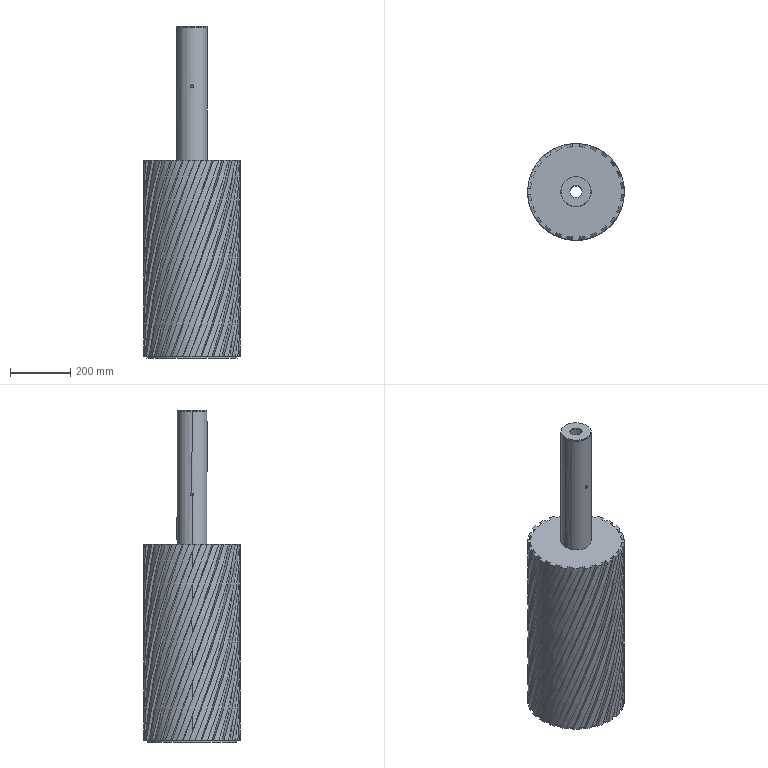Part | SolidWorks | features ICE 12, CirPattern 1, Extrusion 1, Helix 1, Sweep 1 | 3 solids | 135 faces | box 320.001 x 320.001 x 1100 mm | volume 7493467 mm3 | spline 72 | cylinder 54 | plane 9 | commonest cylinder face diameters 300 x32 10 x8 40 x6 100 x4 90 x2 290 x2